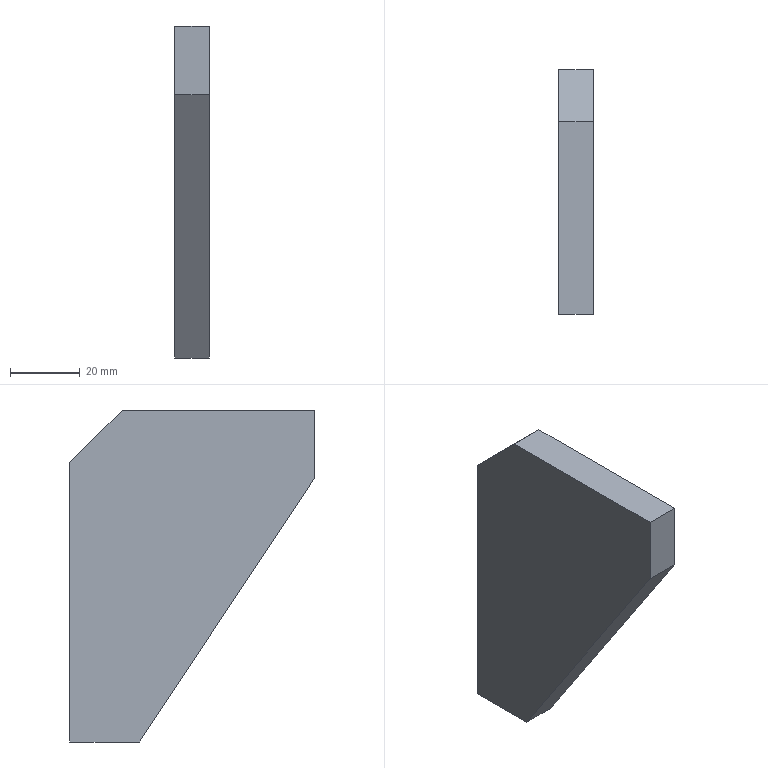Part | STEP file | VD-SYL0380DJ1006_1_5-2_VD-SYL03 | 1 solid | 8 faces | box 10 x 70 x 95 mm | volume 46554 mm3 | plane 8
STEP:
#1=CARTESIAN_POINT('',(0.,0.,-95.));
#2=VERTEX_POINT('',#1);
#3=CARTESIAN_POINT('',(0.,-20.,-95.));
#4=VERTEX_POINT('',#3);
#5=CARTESIAN_POINT('',(0.,0.,-95.));
#6=DIRECTION('',(0.,-1.,0.));
#7=VECTOR('',#6,1000.);
#8=LINE('',#5,#7);
#9=EDGE_CURVE('',#2,#4,#8,.T.);
#10=ORIENTED_EDGE('',*,*,#9,.T.);
#11=CARTESIAN_POINT('',(0.,-70.,-19.716));
#12=VERTEX_POINT('',#11);
#13=CARTESIAN_POINT('',(0.,-20.,-95.));
#14=DIRECTION('',(0.,-0.5532,0.833));
#15=VECTOR('',#14,1000.);
#16=LINE('',#13,#15);
#17=EDGE_CURVE('',#4,#12,#16,.T.);
#18=ORIENTED_EDGE('',*,*,#17,.T.);
#19=CARTESIAN_POINT('',(0.,-70.,0.));
#20=VERTEX_POINT('',#19);
#21=CARTESIAN_POINT('',(0.,-70.,-19.716));
#22=DIRECTION('',(0.,0.,1.));
#23=VECTOR('',#22,1000.);
#24=LINE('',#21,#23);
#25=EDGE_CURVE('',#12,#20,#24,.T.);
#26=ORIENTED_EDGE('',*,*,#25,.T.);
#27=CARTESIAN_POINT('',(0.,-15.,0.));
#28=VERTEX_POINT('',#27);
#29=CARTESIAN_POINT('',(0.,-70.,0.));
#30=DIRECTION('',(0.,1.,0.));
#31=VECTOR('',#30,1000.);
#32=LINE('',#29,#31);
#33=EDGE_CURVE('',#20,#28,#32,.T.);
#34=ORIENTED_EDGE('',*,*,#33,.T.);
#35=CARTESIAN_POINT('',(0.,0.,-15.));
#36=VERTEX_POINT('',#35);
#37=CARTESIAN_POINT('',(0.,-15.,0.));
#38=DIRECTION('',(0.,0.7071,-0.7071));
#39=VECTOR('',#38,1000.);
#40=LINE('',#37,#39);
#41=EDGE_CURVE('',#28,#36,#40,.T.);
#42=ORIENTED_EDGE('',*,*,#41,.T.);
#43=CARTESIAN_POINT('',(0.,0.,-15.));
#44=DIRECTION('',(0.,0.,-1.));
#45=VECTOR('',#44,1000.);
#46=LINE('',#43,#45);
#47=EDGE_CURVE('',#36,#2,#46,.T.);
#48=ORIENTED_EDGE('',*,*,#47,.T.);
#49=EDGE_LOOP('',(#10,#18,#26,#34,#42,#48));
#50=FACE_OUTER_BOUND('',#49,.T.);
#51=CARTESIAN_POINT('',(0.,0.,0.));
#52=DIRECTION('',(1.,0.,0.));
#53=DIRECTION('',(0.,1.,0.));
#54=AXIS2_PLACEMENT_3D('',#51,#52,#53);
#55=PLANE('',#54);
#56=ADVANCED_FACE('',(#50),#55,.F.);
#57=CARTESIAN_POINT('',(10.,-15.,0.));
#58=VERTEX_POINT('',#57);
#59=CARTESIAN_POINT('',(10.,-70.,0.));
#60=VERTEX_POINT('',#59);
#61=CARTESIAN_POINT('',(10.,-15.,0.));
#62=DIRECTION('',(0.,-1.,0.));
#63=VECTOR('',#62,1000.);
#64=LINE('',#61,#63);
#65=EDGE_CURVE('',#58,#60,#64,.T.);
#66=ORIENTED_EDGE('',*,*,#65,.T.);
#67=CARTESIAN_POINT('',(10.,-70.,-19.716));
#68=VERTEX_POINT('',#67);
#69=CARTESIAN_POINT('',(10.,-70.,0.));
#70=DIRECTION('',(0.,0.,-1.));
#71=VECTOR('',#70,1000.);
#72=LINE('',#69,#71);
#73=EDGE_CURVE('',#60,#68,#72,.T.);
#74=ORIENTED_EDGE('',*,*,#73,.T.);
#75=CARTESIAN_POINT('',(10.,-20.,-95.));
#76=VERTEX_POINT('',#75);
#77=CARTESIAN_POINT('',(10.,-70.,-19.716));
#78=DIRECTION('',(0.,0.5532,-0.833));
#79=VECTOR('',#78,1000.);
#80=LINE('',#77,#79);
#81=EDGE_CURVE('',#68,#76,#80,.T.);
#82=ORIENTED_EDGE('',*,*,#81,.T.);
#83=CARTESIAN_POINT('',(10.,0.,-95.));
#84=VERTEX_POINT('',#83);
#85=CARTESIAN_POINT('',(10.,-20.,-95.));
#86=DIRECTION('',(0.,1.,0.));
#87=VECTOR('',#86,1000.);
#88=LINE('',#85,#87);
#89=EDGE_CURVE('',#76,#84,#88,.T.);
#90=ORIENTED_EDGE('',*,*,#89,.T.);
#91=CARTESIAN_POINT('',(10.,0.,-15.));
#92=VERTEX_POINT('',#91);
#93=CARTESIAN_POINT('',(10.,0.,-95.));
#94=DIRECTION('',(0.,0.,1.));
#95=VECTOR('',#94,1000.);
#96=LINE('',#93,#95);
#97=EDGE_CURVE('',#84,#92,#96,.T.);
#98=ORIENTED_EDGE('',*,*,#97,.T.);
#99=CARTESIAN_POINT('',(10.,0.,-15.));
#100=DIRECTION('',(0.,-0.7071,0.7071));
#101=VECTOR('',#100,1000.);
#102=LINE('',#99,#101);
#103=EDGE_CURVE('',#92,#58,#102,.T.);
#104=ORIENTED_EDGE('',*,*,#103,.T.);
#105=EDGE_LOOP('',(#66,#74,#82,#90,#98,#104));
#106=FACE_OUTER_BOUND('',#105,.T.);
#107=CARTESIAN_POINT('',(10.,0.,0.));
#108=DIRECTION('',(1.,0.,0.));
#109=DIRECTION('',(0.,1.,0.));
#110=AXIS2_PLACEMENT_3D('',#107,#108,#109);
#111=PLANE('',#110);
#112=ADVANCED_FACE('',(#106),#111,.T.);
#113=ORIENTED_EDGE('',*,*,#9,.F.);
#114=CARTESIAN_POINT('',(0.,0.,-95.));
#115=DIRECTION('',(1.,0.,0.));
#116=VECTOR('',#115,1000.);
#117=LINE('',#114,#116);
#118=EDGE_CURVE('',#2,#84,#117,.T.);
#119=ORIENTED_EDGE('',*,*,#118,.T.);
#120=ORIENTED_EDGE('',*,*,#89,.F.);
#121=CARTESIAN_POINT('',(0.,-20.,-95.));
#122=DIRECTION('',(1.,0.,0.));
#123=VECTOR('',#122,1000.);
#124=LINE('',#121,#123);
#125=EDGE_CURVE('',#4,#76,#124,.T.);
#126=ORIENTED_EDGE('',*,*,#125,.F.);
#127=EDGE_LOOP('',(#113,#119,#120,#126));
#128=FACE_OUTER_BOUND('',#127,.T.);
#129=CARTESIAN_POINT('',(0.,-20.,-95.));
#130=DIRECTION('',(0.,0.,-1.));
#131=DIRECTION('',(0.,-1.,0.));
#132=AXIS2_PLACEMENT_3D('',#129,#130,#131);
#133=PLANE('',#132);
#134=ADVANCED_FACE('',(#128),#133,.T.);
#135=ORIENTED_EDGE('',*,*,#47,.F.);
#136=CARTESIAN_POINT('',(0.,0.,-15.));
#137=DIRECTION('',(1.,0.,0.));
#138=VECTOR('',#137,1000.);
#139=LINE('',#136,#138);
#140=EDGE_CURVE('',#36,#92,#139,.T.);
#141=ORIENTED_EDGE('',*,*,#140,.T.);
#142=ORIENTED_EDGE('',*,*,#97,.F.);
#143=ORIENTED_EDGE('',*,*,#118,.F.);
#144=EDGE_LOOP('',(#135,#141,#142,#143));
#145=FACE_OUTER_BOUND('',#144,.T.);
#146=CARTESIAN_POINT('',(0.,0.,-95.));
#147=DIRECTION('',(0.,1.,0.));
#148=DIRECTION('',(1.,0.,0.));
#149=AXIS2_PLACEMENT_3D('',#146,#147,#148);
#150=PLANE('',#149);
#151=ADVANCED_FACE('',(#145),#150,.T.);
#152=ORIENTED_EDGE('',*,*,#41,.F.);
#153=CARTESIAN_POINT('',(10.,-15.,0.));
#154=DIRECTION('',(-1.,0.,0.));
#155=VECTOR('',#154,1000.);
#156=LINE('',#153,#155);
#157=EDGE_CURVE('',#58,#28,#156,.T.);
#158=ORIENTED_EDGE('',*,*,#157,.F.);
#159=ORIENTED_EDGE('',*,*,#103,.F.);
#160=ORIENTED_EDGE('',*,*,#140,.F.);
#161=EDGE_LOOP('',(#152,#158,#159,#160));
#162=FACE_OUTER_BOUND('',#161,.T.);
#163=CARTESIAN_POINT('',(0.,0.,-15.));
#164=DIRECTION('',(0.,0.7071,0.7071));
#165=DIRECTION('',(1.,0.,0.));
#166=AXIS2_PLACEMENT_3D('',#163,#164,#165);
#167=PLANE('',#166);
#168=ADVANCED_FACE('',(#162),#167,.T.);
#169=ORIENTED_EDGE('',*,*,#33,.F.);
#170=CARTESIAN_POINT('',(0.,-70.,0.));
#171=DIRECTION('',(1.,0.,0.));
#172=VECTOR('',#171,1000.);
#173=LINE('',#170,#172);
#174=EDGE_CURVE('',#20,#60,#173,.T.);
#175=ORIENTED_EDGE('',*,*,#174,.T.);
#176=ORIENTED_EDGE('',*,*,#65,.F.);
#177=ORIENTED_EDGE('',*,*,#157,.T.);
#178=EDGE_LOOP('',(#169,#175,#176,#177));
#179=FACE_OUTER_BOUND('',#178,.T.);
#180=CARTESIAN_POINT('',(0.,-15.,0.));
#181=DIRECTION('',(0.,0.,1.));
#182=DIRECTION('',(1.,0.,0.));
#183=AXIS2_PLACEMENT_3D('',#180,#181,#182);
#184=PLANE('',#183);
#185=ADVANCED_FACE('',(#179),#184,.T.);
#186=ORIENTED_EDGE('',*,*,#25,.F.);
#187=CARTESIAN_POINT('',(0.,-70.,-19.716));
#188=DIRECTION('',(1.,0.,0.));
#189=VECTOR('',#188,1000.);
#190=LINE('',#187,#189);
#191=EDGE_CURVE('',#12,#68,#190,.T.);
#192=ORIENTED_EDGE('',*,*,#191,.T.);
#193=ORIENTED_EDGE('',*,*,#73,.F.);
#194=ORIENTED_EDGE('',*,*,#174,.F.);
#195=EDGE_LOOP('',(#186,#192,#193,#194));
#196=FACE_OUTER_BOUND('',#195,.T.);
#197=CARTESIAN_POINT('',(0.,-70.,0.));
#198=DIRECTION('',(0.,-1.,0.));
#199=DIRECTION('',(0.,0.,-1.));
#200=AXIS2_PLACEMENT_3D('',#197,#198,#199);
#201=PLANE('',#200);
#202=ADVANCED_FACE('',(#196),#201,.T.);
#203=ORIENTED_EDGE('',*,*,#17,.F.);
#204=ORIENTED_EDGE('',*,*,#125,.T.);
#205=ORIENTED_EDGE('',*,*,#81,.F.);
#206=ORIENTED_EDGE('',*,*,#191,.F.);
#207=EDGE_LOOP('',(#203,#204,#205,#206));
#208=FACE_OUTER_BOUND('',#207,.T.);
#209=CARTESIAN_POINT('',(0.,-70.,-19.716));
#210=DIRECTION('',(0.,-0.833,-0.5532));
#211=DIRECTION('',(0.,0.5532,-0.833));
#212=AXIS2_PLACEMENT_3D('',#209,#210,#211);
#213=PLANE('',#212);
#214=ADVANCED_FACE('',(#208),#213,.T.);
#215=CLOSED_SHELL('',(#56,#112,#134,#151,#168,#185,#202,#214));
#216=MANIFOLD_SOLID_BREP('',#215);
#217=CARTESIAN_POINT('',(0.,0.,0.));
#218=DIRECTION('',(0.,0.,1.));
#219=DIRECTION('',(1.,0.,0.));
#220=AXIS2_PLACEMENT_3D('',#217,#218,#219);
#221=(LENGTH_UNIT()NAMED_UNIT(*)SI_UNIT(.MILLI.,.METRE.));
#222=UNCERTAINTY_MEASURE_WITH_UNIT(LENGTH_MEASURE(0.00001),#221,'','');
#223=(NAMED_UNIT(*)PLANE_ANGLE_UNIT()SI_UNIT($,.RADIAN.));
#224=(NAMED_UNIT(*)SI_UNIT($,.STERADIAN.)SOLID_ANGLE_UNIT());
#225=(GEOMETRIC_REPRESENTATION_CONTEXT(3)GLOBAL_UNCERTAINTY_ASSIGNED_CONTEXT((#222))GLOBAL_UNIT_ASSIGNED_CONTEXT((#221,#223,#224))REPRESENTATION_CONTEXT('',''));
#226=ADVANCED_BREP_SHAPE_REPRESENTATION('',(#216,#220),#225);